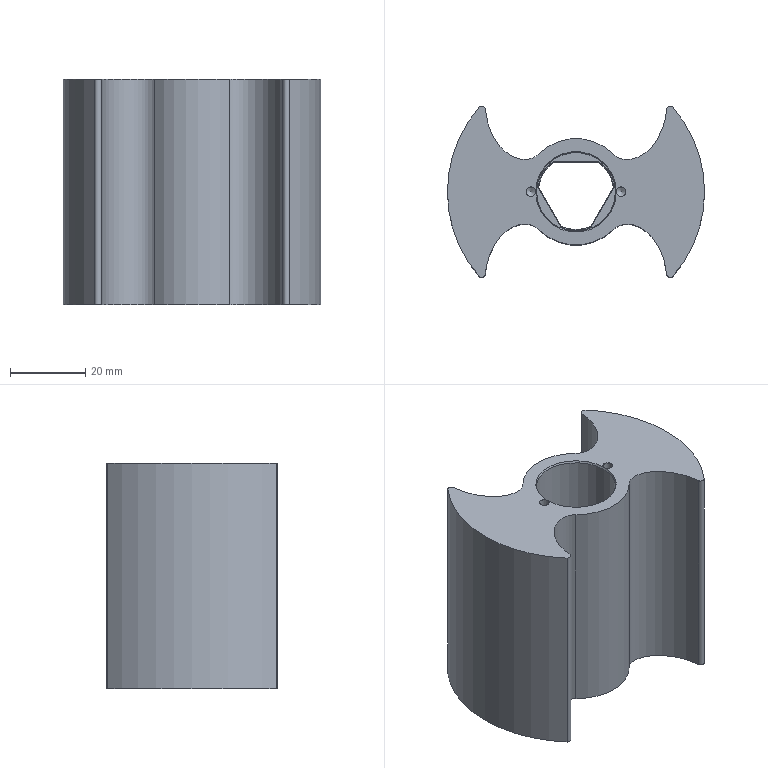NC program | NX | posted with a generic post | part box 68.489 x 45.577 x 60 mm
Whole program:
N10 G17 G21 G94 G90
(DRILLING_COPY_1 , TOOL : ZXZ)
N12 T01 M6
N14 G54
N16 G17 G0 G90 X-12. Y0. S5000 M3
N18 G43 Z30. H1
N20 G94 G81 G98 Z-1. F250. R3.
N22 X12.
N24 G80
N26 G0 X12. Y0. Z30.
N28 M5
(DRILLING_COPY_1_COPY , TOOL : 2.5ZT)
N30 T12 M6
N32 G54
N34 G17 G0 G90 X-12. Y0. S2000 M3
N36 G43 Z30. H12
N38 G94 G83 G98 Z-4.751 F120. Q2. R3.
N40 X12.
N42 G80
N44 G0 X12. Y0. Z30.
N46 M5
(ZLEVEL_PROFILE_COPY_1 , TOOL : D12)
N48 M6
N50 G54
N52 G17 G0 G90 X-0.209 Y-3.338 S3000 M3
N54 G43 Z30. H12
N56 Z-12.2
N58 G94 G1 X0. Y-3.7 Z-12.211 F1000.
N60 X3.204 Y1.85 Z-12.379
N62 X-3.204 Z-12.547
N64 X0. Y-3.7 Z-12.714
N66 X3.204 Y1.85 Z-12.882
N68 X-3.204 Z-13.05
N70 X0. Y-3.7 Z-13.218
N72 X3.204 Y1.85 Z-13.386
N74 X-3.204 Z-13.553
N76 X0. Y-3.7 Z-13.721
N78 X3.204 Y1.85 Z-13.889
N80 X-3.204 Z-14.057
N82 X0. Y-3.7 Z-14.225
N84 X3.204 Y1.85 Z-14.393
N86 X-3.204 Z-14.56
N88 X0. Y-3.7 Z-14.728
N90 X3.204 Y1.85 Z-14.896
N92 X-3.204 Z-15.064
N94 X0. Y-3.7 Z-15.232
N96 X3.204 Y1.85 Z-15.399
N98 X-3.204 F1800.
N100 X0. Y-3.7
N102 X3.204 Y1.85
N104 X-3.143 Z-15.51
N106 X-3.023 Y1.536 Z-15.518
N108 X-0.696 Y-2.495 Z-15.599
N110 X0. Y-3.7
N112 X3.204 Y1.85
N114 X-3.143 Z-15.71
N116 X-3.023 Y1.536 Z-15.717
N118 X-0.696 Y-2.495 Z-15.798
N120 X0. Y-3.7
N122 X3.204 Y1.85
N124 X-3.143 Z-15.909
N126 X-3.023 Y1.536 Z-15.916
N128 X-0.696 Y-2.495 Z-15.998
N130 X0. Y-3.7
N132 X3.204 Y1.85
N134 X-3.143 Z-16.109
N136 X-3.023 Y1.536 Z-16.116
N138 X-0.696 Y-2.495 Z-16.197
N140 X0. Y-3.7
N142 X3.204 Y1.85
N144 X-3.143 Z-16.308
N146 X-3.023 Y1.536 Z-16.315
N148 X-0.696 Y-2.495 Z-16.397
N150 X0. Y-3.7
N152 X3.204 Y1.85
N154 X-3.143 Z-16.507
N156 X-3.023 Y1.536 Z-16.515
N158 X-0.696 Y-2.495 Z-16.596
N160 X0. Y-3.7
N162 X3.204 Y1.85
N164 X-3.143 Z-16.707
N166 X-3.023 Y1.536 Z-16.714
N168 X-0.696 Y-2.495 Z-16.795
N170 X0. Y-3.7
N172 X3.204 Y1.85
N174 X-3.143 Z-16.906
N176 X-3.023 Y1.536 Z-16.914
N178 X-0.696 Y-2.495 Z-16.995
N180 X0. Y-3.7
N182 X3.204 Y1.85
N184 X-3.143 Z-17.106
N186 X-3.023 Y1.536 Z-17.113
N188 X-0.696 Y-2.495 Z-17.194
N190 X0. Y-3.7
N192 X3.204 Y1.85
N194 X-3.143 Z-17.305
N196 X-3.023 Y1.536 Z-17.313
N198 X-0.696 Y-2.495 Z-17.394
N200 X0. Y-3.7
N202 X3.204 Y1.85
N204 X-3.143 Z-17.505
N206 X-3.023 Y1.536 Z-17.512
N208 X-0.696 Y-2.495 Z-17.593
N210 X0. Y-3.7
N212 X3.204 Y1.85
N214 X-3.143 Z-17.704
N216 X-3.023 Y1.536 Z-17.711
N218 X-0.696 Y-2.495 Z-17.793
N220 X0. Y-3.7
N222 X3.204 Y1.85
N224 X-3.143 Z-17.903
N226 X-3.023 Y1.536 Z-17.911
N228 X-0.696 Y-2.495 Z-17.992
N230 X0. Y-3.7
N232 X3.204 Y1.85
N234 X-3.143 Z-18.103
N236 X-3.023 Y1.536 Z-18.11
N238 X-0.696 Y-2.495 Z-18.192
N240 X0. Y-3.7
N242 X3.204 Y1.85
N244 X-3.143 Z-18.302
N246 X-3.023 Y1.536 Z-18.31
N248 X-0.696 Y-2.495 Z-18.391
N250 X0. Y-3.7
N252 X3.204 Y1.85
N254 X-3.143 Z-18.502
N256 X-3.023 Y1.536 Z-18.509
N258 X-0.696 Y-2.495 Z-18.59
N260 X0. Y-3.7
N262 X3.204 Y1.85
N264 X-3.143 Z-18.701
N266 X-3.023 Y1.536 Z-18.709
N268 X-0.696 Y-2.495 Z-18.79
N270 X0. Y-3.7
N272 X3.204 Y1.85
N274 X-3.143 Z-18.901
N276 X-3.023 Y1.536 Z-18.908
N278 X-0.696 Y-2.495 Z-18.989
N280 X0. Y-3.7
N282 X3.204 Y1.85
N284 X-3.143 Z-19.1
N286 X-3.023 Y1.536 Z-19.107
N288 X-0.696 Y-2.495 Z-19.189
N290 X0. Y-3.7
N292 X3.204 Y1.85
N294 X-3.143 Z-19.299
N296 X-3.023 Y1.536 Z-19.307
N298 X-0.696 Y-2.495 Z-19.388
N300 X0. Y-3.7
N302 X3.204 Y1.85
N304 X-3.143 Z-19.499
N306 X-3.023 Y1.536 Z-19.506
N308 X-0.696 Y-2.495 Z-19.588
N310 X0. Y-3.7
N312 X3.204 Y1.85
N314 X-3.143 Z-19.698
N316 X-3.023 Y1.536 Z-19.706
N318 X-0.696 Y-2.495 Z-19.787
N320 X0. Y-3.7
N322 X3.204 Y1.85
N324 X-3.143 Z-19.898
N326 X-3.023 Y1.536 Z-19.905
N328 X-0.696 Y-2.495 Z-19.986
N330 X0. Y-3.7
N332 X3.204 Y1.85
N334 X-3.143 Z-20.097
N336 X-3.023 Y1.536 Z-20.105
N338 X-0.696 Y-2.495 Z-20.186
N340 X0. Y-3.7
N342 X3.204 Y1.85
N344 X-3.143 Z-20.297
N346 X-3.023 Y1.536 Z-20.304
N348 X-0.696 Y-2.495 Z-20.385
N350 X0. Y-3.7
N352 X3.204 Y1.85
N354 X-3.143 Z-20.496
N356 X-3.023 Y1.536 Z-20.503
N358 X-0.696 Y-2.495 Z-20.585
N360 X0. Y-3.7
N362 X3.204 Y1.85
N364 X-3.143 Z-20.696
N366 X-3.023 Y1.536 Z-20.703
N368 X-0.696 Y-2.495 Z-20.784
N370 X0. Y-3.7
N372 X3.204 Y1.85
N374 X-3.143 Z-20.895
N376 X-3.023 Y1.536 Z-20.902
N378 X-0.696 Y-2.495 Z-20.984
N380 X0. Y-3.7
N382 X3.204 Y1.85
N384 X-3.143 Z-21.094
N386 X-3.023 Y1.536 Z-21.102
N388 X-0.696 Y-2.495 Z-21.183
N390 X0. Y-3.7
N392 X3.204 Y1.85
N394 X-3.143 Z-21.294
N396 X-3.023 Y1.536 Z-21.301
N398 X-0.696 Y-2.495 Z-21.382
N400 X0. Y-3.7
N402 X3.204 Y1.85
N404 X-3.143 Z-21.493
N406 X-3.023 Y1.536 Z-21.501
N408 X-0.696 Y-2.495 Z-21.582
N410 X0. Y-3.7
N412 X3.204 Y1.85
N414 X-3.143 Z-21.693
N416 X-3.023 Y1.536 Z-21.7
N418 X-0.696 Y-2.495 Z-21.781
N420 X0. Y-3.7
N422 X3.204 Y1.85
N424 X-3.143 Z-21.892
N426 X-3.023 Y1.536 Z-21.9
N428 X-0.696 Y-2.495 Z-21.981
N430 X0. Y-3.7
N432 X3.204 Y1.85
N434 X-3.143 Z-22.092
N436 X-3.023 Y1.536 Z-22.099
N438 X-0.696 Y-2.495 Z-22.18
N440 X0. Y-3.7
N442 X3.204 Y1.85
N444 X-3.143 Z-22.291
N446 X-3.023 Y1.536 Z-22.298
N448 X-0.696 Y-2.495 Z-22.38
N450 X0. Y-3.7
N452 X3.204 Y1.85
N454 X-3.143 Z-22.49
N456 X-3.023 Y1.536 Z-22.498
N458 X-0.696 Y-2.495 Z-22.579
N460 X0. Y-3.7
N462 X3.204 Y1.85
N464 X-3.143 Z-22.69
N466 X-3.023 Y1.536 Z-22.697
N468 X-0.696 Y-2.495 Z-22.779
N470 X0. Y-3.7
N472 X3.204 Y1.85
N474 X-3.143 Z-22.889
N476 X-3.023 Y1.536 Z-22.897
N478 X-0.696 Y-2.495 Z-22.978
N480 X0. Y-3.7
N482 X3.204 Y1.85
N484 X-3.143 Z-23.089
N486 X-3.023 Y1.536 Z-23.096
N488 X-0.696 Y-2.495 Z-23.177
N490 X0. Y-3.7
N492 X3.204 Y1.85
N494 X-3.143 Z-23.288
N496 X-3.023 Y1.536 Z-23.296
N498 X-0.696 Y-2.495 Z-23.377
N500 X0. Y-3.7
N502 X3.204 Y1.85
N504 X-3.143 Z-23.488
N506 X-3.023 Y1.536 Z-23.495
N508 X-0.696 Y-2.495 Z-23.576
N510 X0. Y-3.7
N512 X3.204 Y1.85
N514 X-3.143 Z-23.687
N516 X-3.023 Y1.536 Z-23.694
N518 X-0.696 Y-2.495 Z-23.776
N520 X0. Y-3.7
N522 X3.204 Y1.85
N524 X-3.143 Z-23.887
N526 X-3.023 Y1.536 Z-23.894
N528 X-0.696 Y-2.495 Z-23.975
N530 X0. Y-3.7
N532 X3.204 Y1.85
N534 X-3.143 Z-24.086
N536 X-3.023 Y1.536 Z-24.093
N538 X-0.696 Y-2.495 Z-24.175
N540 X0. Y-3.7
N542 X3.204 Y1.85
N544 X-3.143 Z-24.285
N546 X-3.023 Y1.536 Z-24.293
N548 X-0.696 Y-2.495 Z-24.374
N550 X0. Y-3.7
N552 X3.204 Y1.85
N554 X-3.143 Z-24.485
N556 X-3.023 Y1.536 Z-24.492
N558 X-0.696 Y-2.495 Z-24.573
N560 X0. Y-3.7
N562 X3.204 Y1.85
N564 X-3.143 Z-24.684
N566 X-3.023 Y1.536 Z-24.692
N568 X-0.696 Y-2.495 Z-24.773
N570 X0. Y-3.7
N572 X3.204 Y1.85
N574 X-3.143 Z-24.884
N576 X-3.023 Y1.536 Z-24.891
N578 X-0.696 Y-2.495 Z-24.972
N580 X0. Y-3.7
N582 X3.204 Y1.85
N584 X-3.143 Z-25.083
N586 X-3.023 Y1.536 Z-25.091
N588 X-0.696 Y-2.495 Z-25.172
N590 X0. Y-3.7
N592 X3.204 Y1.85
N594 X-3.143 Z-25.283
N596 X-3.023 Y1.536 Z-25.29
N598 X-0.696 Y-2.495 Z-25.371
N600 X0. Y-3.7
N602 X3.204 Y1.85
N604 X-3.143 Z-25.482
N606 X-3.023 Y1.536 Z-25.489
N608 X-0.696 Y-2.495 Z-25.571
N610 X0. Y-3.7
N612 X3.204 Y1.85
N614 X-3.143 Z-25.681
N616 X-3.023 Y1.536 Z-25.689
N618 X-0.696 Y-2.495 Z-25.77
N620 X0. Y-3.7
N622 X3.204 Y1.85
N624 X-3.143 Z-25.881
N626 X-3.023 Y1.536 Z-25.888
N628 X-0.696 Y-2.495 Z-25.969
N630 X0. Y-3.7
N632 X3.204 Y1.85
N634 X-3.143 Z-26.08
N636 X-3.023 Y1.536 Z-26.088
N638 X-0.696 Y-2.495 Z-26.169
N640 X0. Y-3.7
N642 X3.204 Y1.85
N644 X-3.143 Z-26.28
N646 X-3.023 Y1.536 Z-26.287
N648 X-0.696 Y-2.495 Z-26.368
N650 X0. Y-3.7
N652 X3.204 Y1.85
N654 X-3.143 Z-26.479
N656 X-3.023 Y1.536 Z-26.487
N658 X-0.696 Y-2.495 Z-26.568
N660 X0. Y-3.7
N662 X3.204 Y1.85
N664 X-3.143 Z-26.679
N666 X-3.023 Y1.536 Z-26.686
N668 X-0.696 Y-2.495 Z-26.767
N670 X0. Y-3.7
N672 X3.204 Y1.85
N674 X-3.143 Z-26.878
N676 X-3.023 Y1.536 Z-26.885
N678 X-0.696 Y-2.495 Z-26.967
N680 X0. Y-3.7
N682 X3.204 Y1.85
N684 X-3.143 Z-27.077
N686 X-3.023 Y1.536 Z-27.085
N688 X-0.696 Y-2.495 Z-27.166
N690 X0. Y-3.7
N692 X3.204 Y1.85
N694 X-3.143 Z-27.277
N696 X-3.023 Y1.536 Z-27.284
N698 X-0.696 Y-2.495 Z-27.366
N700 X0. Y-3.7
N702 X3.204 Y1.85
N704 X-3.143 Z-27.476
N706 X-3.023 Y1.536 Z-27.484
N708 X-0.696 Y-2.495 Z-27.565
N710 X0. Y-3.7
N712 X3.204 Y1.85
N714 X-3.143 Z-27.676
N716 X-3.023 Y1.536 Z-27.683
N718 X-0.696 Y-2.495 Z-27.764
N720 X0. Y-3.7
N722 X3.204 Y1.85
N724 X-3.143 Z-27.875
N726 X-3.023 Y1.536 Z-27.883
N728 X-0.696 Y-2.495 Z-27.964
N730 X0. Y-3.7
N732 X3.204 Y1.85
N734 X-3.143 Z-28.075
N736 X-3.023 Y1.536 Z-28.082
N738 X-0.696 Y-2.495 Z-28.163
N740 X0. Y-3.7
N742 X3.204 Y1.85
N744 X-3.143 Z-28.274
N746 X-3.023 Y1.536 Z-28.281
N748 X-0.696 Y-2.495 Z-28.363
N750 X0. Y-3.7
N752 X3.204 Y1.85
N754 X-3.143 Z-28.474
N756 X-3.023 Y1.536 Z-28.481
N758 X-0.696 Y-2.495 Z-28.562
N760 X0. Y-3.7
N762 X3.204 Y1.85
N764 X-3.143 Z-28.673
N766 X-3.023 Y1.536 Z-28.68
N768 X-0.696 Y-2.495 Z-28.762
N770 X0. Y-3.7
N772 X3.204 Y1.85
N774 X-3.143 Z-28.872
N776 X-3.023 Y1.536 Z-28.88
N778 X-0.696 Y-2.495 Z-28.961
N780 X0. Y-3.7
N782 X3.204 Y1.85
N784 X-3.143 Z-29.072
N786 X-3.023 Y1.536 Z-29.079
N788 X-0.696 Y-2.495 Z-29.16
N790 X0. Y-3.7
N792 X3.204 Y1.85
N794 X-3.143 Z-29.271
N796 X-3.023 Y1.536 Z-29.279
N798 X-0.696 Y-2.495 Z-29.36
N800 X0. Y-3.7
N802 X3.204 Y1.85
N804 X-3.143 Z-29.471
N806 X-3.023 Y1.536 Z-29.478
N808 X-0.696 Y-2.495 Z-29.559
N810 X0. Y-3.7
N812 X3.204 Y1.85
N814 X-3.143 Z-29.67
N816 X-3.023 Y1.536 Z-29.678
N818 X-0.696 Y-2.495 Z-29.759
N820 X0. Y-3.7
N822 X3.204 Y1.85
N824 X-3.143 Z-29.87
N826 X-3.023 Y1.536 Z-29.877
N828 X-0.696 Y-2.495 Z-29.958
N830 X0. Y-3.7
N832 X3.204 Y1.85
N834 X-3.143 Z-30.069
N836 X-3.023 Y1.536 Z-30.076
N838 X-0.696 Y-2.495 Z-30.158
N840 X0. Y-3.7
N842 X3.204 Y1.85
N844 X-3.143 Z-30.268
N846 X-3.023 Y1.536 Z-30.276
N848 X-0.696 Y-2.495 Z-30.357
N850 X0. Y-3.7
N852 X3.204 Y1.85
N854 X-3.143 Z-30.468
N856 X-3.023 Y1.536 Z-30.475
N858 X-0.696 Y-2.495 Z-30.556
N860 X0. Y-3.7
N862 X3.204 Y1.85
N864 X-3.143 Z-30.667
N866 X-3.023 Y1.536 Z-30.675
N868 X-0.696 Y-2.495 Z-30.756
N870 X0. Y-3.7
N872 X3.204 Y1.85
N874 X-3.143 Z-30.867
N876 X-3.023 Y1.536 Z-30.874
N878 X-0.696 Y-2.495 Z-30.955
N880 X0. Y-3.7
N882 X3.204 Y1.85
N884 X-3.143 Z-31.066
N886 X-3.023 Y1.536 Z-31.074
N888 X-0.696 Y-2.495 Z-31.155
N890 X0. Y-3.7
N892 X3.204 Y1.85
N894 X-3.143 Z-31.266
N896 X-3.023 Y1.536 Z-31.273
N898 X-0.696 Y-2.495 Z-31.354
N900 X0. Y-3.7
N902 X3.204 Y1.85
N904 X-3.143 Z-31.465
N906 X-3.023 Y1.536 Z-31.472
N908 X-0.696 Y-2.495 Z-31.554
N910 X0. Y-3.7
N912 X3.204 Y1.85
N914 X-3.143 Z-31.664
N916 X-3.023 Y1.536 Z-31.672
N918 X-0.696 Y-2.495 Z-31.753
N920 X0. Y-3.7
N922 X3.204 Y1.85
N924 X-3.143 Z-31.864
N926 X-3.023 Y1.536 Z-31.871
N928 X-0.696 Y-2.495 Z-31.953
N930 X0. Y-3.7
N932 X3.204 Y1.85
N934 X-3.143 Z-32.063
N936 X-3.023 Y1.536 Z-32.071
N938 X-0.696 Y-2.495 Z-32.152
N940 X0. Y-3.7
N942 X3.204 Y1.85
N944 X-3.143 Z-32.263
N946 X-3.023 Y1.536 Z-32.27
N948 X-0.696 Y-2.495 Z-32.351
N950 X0. Y-3.7
N952 X3.204 Y1.85
N954 X-3.143 Z-32.462
N956 X-3.023 Y1.536 Z-32.47
N958 X-0.696 Y-2.495 Z-32.551
N960 X0. Y-3.7
N962 X3.204 Y1.85
N964 X-3.143 Z-32.662
N966 X-3.023 Y1.536 Z-32.669
N968 X-0.696 Y-2.495 Z-32.75
N970 X0. Y-3.7
N972 X3.204 Y1.85
N974 X-3.143 Z-32.861
N976 X-3.023 Y1.536 Z-32.868
N978 X-0.696 Y-2.495 Z-32.95
N980 X0. Y-3.7
N982 X3.204 Y1.85
N984 X-3.143 Z-33.061
N986 X-3.023 Y1.536 Z-33.068
N988 X-0.696 Y-2.495 Z-33.149
N990 X0. Y-3.7
N992 X3.204 Y1.85
N994 X-3.143 Z-33.26
N996 X-3.023 Y1.536 Z-33.267
N998 X-0.696 Y-2.495 Z-33.349
N1000 X0. Y-3.7
N1002 X3.204 Y1.85
N1004 X-3.143 Z-33.459
N1006 X-3.023 Y1.536 Z-33.467
N1008 X-0.696 Y-2.495 Z-33.548
N1010 X0. Y-3.7
N1012 X3.204 Y1.85
N1014 X-3.143 Z-33.659
N1016 X-3.023 Y1.536 Z-33.666
N1018 X-0.696 Y-2.495 Z-33.747
N1020 X0. Y-3.7
N1022 X3.204 Y1.85
N1024 X-3.143 Z-33.858
N1026 X-3.023 Y1.536 Z-33.866
N1028 X-0.696 Y-2.495 Z-33.947
N1030 X0. Y-3.7
N1032 X3.204 Y1.85
N1034 X-3.143 Z-34.058
N1036 X-3.023 Y1.536 Z-34.065
N1038 X-0.696 Y-2.495 Z-34.146
N1040 X0. Y-3.7
N1042 X3.204 Y1.85
N1044 X-3.143 Z-34.257
N1046 X-3.023 Y1.536 Z-34.265
N1048 X-0.696 Y-2.495 Z-34.346
N1050 X0. Y-3.7
N1052 X3.204 Y1.85
N1054 X-3.143 Z-34.457
N1056 X-3.023 Y1.536 Z-34.464
N1058 X-0.696 Y-2.495 Z-34.545
N1060 X0. Y-3.7
N1062 X3.204 Y1.85
N1064 X-3.143 Z-34.656
N1066 X-3.023 Y1.536 Z-34.663
N1068 X-0.696 Y-2.495 Z-34.745
N1070 X0. Y-3.7
N1072 X3.204 Y1.85
N1074 X-3.143 Z-34.855
N1076 X-3.023 Y1.536 Z-34.863
N1078 X-0.696 Y-2.495 Z-34.944
N1080 X0. Y-3.7
N1082 X3.204 Y1.85
N1084 X-3.143 Z-35.055
N1086 X-3.023 Y1.536 Z-35.062
N1088 X-0.696 Y-2.495 Z-35.144
N1090 X0. Y-3.7
N1092 X3.204 Y1.85
N1094 X-3.143 Z-35.254
N1096 X-3.023 Y1.536 Z-35.262
N1098 X-0.696 Y-2.495 Z-35.343
N1100 X0. Y-3.7
N1102 X3.204 Y1.85
N1104 X-3.143 Z-35.454
N1106 X-3.023 Y1.536 Z-35.461
N1108 X-0.696 Y-2.495 Z-35.542
N1110 X0. Y-3.7
N1112 X3.204 Y1.85
N1114 X-3.143 Z-35.653
N1116 X-3.023 Y1.536 Z-35.661
N1118 X-0.696 Y-2.495 Z-35.742
N1120 X0. Y-3.7
N1122 X3.204 Y1.85
N1124 X-3.143 Z-35.853
N1126 X-3.023 Y1.536 Z-35.86
N1128 X-0.696 Y-2.495 Z-35.941
N1130 X0. Y-3.7
N1132 X3.204 Y1.85
N1134 X-3.143 Z-36.052
N1136 X-3.023 Y1.536 Z-36.059
N1138 X-0.696 Y-2.495 Z-36.141
N1140 X0. Y-3.7
N1142 X3.204 Y1.85
N1144 X-3.143 Z-36.251
N1146 X-3.023 Y1.536 Z-36.259
N1148 X-0.696 Y-2.495 Z-36.34
N1150 X0. Y-3.7
N1152 X3.204 Y1.85
N1154 X-3.143 Z-36.451
N1156 X-3.023 Y1.536 Z-36.458
N1158 X-0.696 Y-2.495 Z-36.54
N1160 X0. Y-3.7
N1162 X3.204 Y1.85
N1164 X-3.143 Z-36.65
N1166 X-3.023 Y1.536 Z-36.658
N1168 X-0.696 Y-2.495 Z-36.739
N1170 X0. Y-3.7
N1172 X3.204 Y1.85
N1174 X-3.143 Z-36.85
N1176 X-3.023 Y1.536 Z-36.857
N1178 X-0.696 Y-2.495 Z-36.938
N1180 X0. Y-3.7
N1182 X3.204 Y1.85
N1184 X-3.143 Z-37.049
N1186 X-3.023 Y1.536 Z-37.057
N1188 X-0.696 Y-2.495 Z-37.138
N1190 X0. Y-3.7
N1192 X3.204 Y1.85
N1194 X-3.143 Z-37.249
N1196 X-3.023 Y1.536 Z-37.256
N1198 X-0.696 Y-2.495 Z-37.337
N1200 X0. Y-3.7
N1202 X3.204 Y1.85
N1204 X-3.143 Z-37.448
N1206 X-3.023 Y1.536 Z-37.455
N1208 X-0.696 Y-2.495 Z-37.537
N1210 X0. Y-3.7
N1212 X3.204 Y1.85
N1214 X-3.143 Z-37.648
N1216 X-3.023 Y1.536 Z-37.655
N1218 X-0.696 Y-2.495 Z-37.736
N1220 X0. Y-3.7
N1222 X3.204 Y1.85
N1224 X-3.143 Z-37.847
N1226 X-3.023 Y1.536 Z-37.854
N1228 X-0.696 Y-2.495 Z-37.936
N1230 X0. Y-3.7
N1232 X3.204 Y1.85
N1234 X-3.143 Z-38.046
N1236 X-3.023 Y1.536 Z-38.054
N1238 X-0.696 Y-2.495 Z-38.135
N1240 X0. Y-3.7
N1242 X3.204 Y1.85
N1244 X-3.143 Z-38.246
N1246 X-3.023 Y1.536 Z-38.253
N1248 X-0.696 Y-2.495 Z-38.334
N1250 X0. Y-3.7
N1252 X3.204 Y1.85
N1254 X-3.143 Z-38.445
N1256 X-3.023 Y1.536 Z-38.453
N1258 X-0.696 Y-2.495 Z-38.534
N1260 X0. Y-3.7
N1262 X3.204 Y1.85
N1264 X-3.143 Z-38.645
N1266 X-3.023 Y1.536 Z-38.652
N1268 X-0.696 Y-2.495 Z-38.733
N1270 X0. Y-3.7
N1272 X3.204 Y1.85
N1274 X-3.143 Z-38.844
N1276 X-3.023 Y1.536 Z-38.852
N1278 X-0.696 Y-2.495 Z-38.933
N1280 X0. Y-3.7
N1282 X3.204 Y1.85
N1284 X-3.143 Z-39.044
N1286 X-3.023 Y1.536 Z-39.051
N1288 X-0.696 Y-2.495 Z-39.132
N1290 X0. Y-3.7
N1292 X3.204 Y1.85
N1294 X-3.143 Z-39.243
N1296 X-3.023 Y1.536 Z-39.25
N1298 X-0.696 Y-2.495 Z-39.332
N1300 X0. Y-3.7
N1302 X3.204 Y1.85
N1304 X-3.143 Z-39.442
N1306 X-3.023 Y1.536 Z-39.45
N1308 X-0.696 Y-2.495 Z-39.531
N1310 X0. Y-3.7
N1312 X3.204 Y1.85
N1314 X-3.143 Z-39.642
N1316 X-3.023 Y1.536 Z-39.649
N1318 X-0.696 Y-2.495 Z-39.731
N1320 X0. Y-3.7
N1322 X3.204 Y1.85
N1324 X-3.143 Z-39.841
N1326 X-3.023 Y1.536 Z-39.849
N1328 X-0.696 Y-2.495 Z-39.93
N1330 X0. Y-3.7
N1332 X3.204 Y1.85
N1334 X-3.143 Z-40.041
N1336 X-3.023 Y1.536 Z-40.048
N1338 X-0.696 Y-2.495 Z-40.129
N1340 X0. Y-3.7
N1342 X3.204 Y1.85
N1344 X-3.143 Z-40.24
N1346 X-3.023 Y1.536 Z-40.248
N1348 X-0.696 Y-2.495 Z-40.329
N1350 X0. Y-3.7
N1352 X3.204 Y1.85
N1354 X-3.143 Z-40.44
N1356 X-3.023 Y1.536 Z-40.447
N1358 X-0.696 Y-2.495 Z-40.528
N1360 X0. Y-3.7
N1362 X3.204 Y1.85
N1364 X-3.143 Z-40.639
N1366 X-3.023 Y1.536 Z-40.646
N1368 X-0.696 Y-2.495 Z-40.728
N1370 X0. Y-3.7
N1372 X3.204 Y1.85
N1374 X-3.143 Z-40.838
N1376 X-3.023 Y1.536 Z-40.846
N1378 X-0.696 Y-2.495 Z-40.927
N1380 X0. Y-3.7
N1382 X3.204 Y1.85
N1384 X-3.143 Z-41.038
N1386 X-3.023 Y1.536 Z-41.045
N1388 X-0.696 Y-2.495 Z-41.127
N1390 X0. Y-3.7
N1392 X3.204 Y1.85
N1394 X-3.143 Z-41.237
N1396 X-3.023 Y1.536 Z-41.245
N1398 X-0.696 Y-2.495 Z-41.326
N1400 X0. Y-3.7
N1402 X3.204 Y1.85
N1404 X-3.143 Z-41.437
N1406 X-3.023 Y1.536 Z-41.444
N1408 X-0.696 Y-2.495 Z-41.525
N1410 X0. Y-3.7
N1412 X3.204 Y1.85
N1414 X-3.143 Z-41.636
N1416 X-3.023 Y1.536 Z-41.644
N1418 X-0.696 Y-2.495 Z-41.725
N1420 X0. Y-3.7
N1422 X3.204 Y1.85
N1424 X-3.143 Z-41.836
N1426 X-3.023 Y1.536 Z-41.843
N1428 X-0.696 Y-2.495 Z-41.924
N1430 X0. Y-3.7
N1432 X3.204 Y1.85
N1434 X-3.143 Z-42.035
N1436 X-3.023 Y1.536 Z-42.042
N1438 X-0.696 Y-2.495 Z-42.124
N1440 X0. Y-3.7
N1442 X3.204 Y1.85
N1444 X-3.143 Z-42.235
N1446 X-3.023 Y1.536 Z-42.242
N1448 X-0.696 Y-2.495 Z-42.323
N1450 X0. Y-3.7
N1452 X3.204 Y1.85
N1454 X-3.143 Z-42.434
N1456 X-3.023 Y1.536 Z-42.441
N1458 X-0.696 Y-2.495 Z-42.523
N1460 X0. Y-3.7
N1462 X3.204 Y1.85
N1464 X-3.143 Z-42.633
N1466 X-3.023 Y1.536 Z-42.641
N1468 X-0.696 Y-2.495 Z-42.722
N1470 X0. Y-3.7
N1472 X3.204 Y1.85
N1474 X-3.143 Z-42.833
N1476 X-3.023 Y1.536 Z-42.84
N1478 X-0.696 Y-2.495 Z-42.921
N1480 X0. Y-3.7
N1482 X3.204 Y1.85
N1484 X-3.143 Z-43.032
N1486 X-3.023 Y1.536 Z-43.04
N1488 X-0.696 Y-2.495 Z-43.121
N1490 X0. Y-3.7
N1492 X3.204 Y1.85
N1494 X-3.143 Z-43.232
N1496 X-3.023 Y1.536 Z-43.239
N1498 X-0.696 Y-2.495 Z-43.32
N1500 X0. Y-3.7
N1502 X3.204 Y1.85
N1504 X-3.143 Z-43.431
N1506 X-3.023 Y1.536 Z-43.439
N1508 X-0.696 Y-2.495 Z-43.52
N1510 X0. Y-3.7
N1512 X3.204 Y1.85
N1514 X-3.143 Z-43.631
N1516 X-3.023 Y1.536 Z-43.638
N1518 X-0.696 Y-2.495 Z-43.719
N1520 X0. Y-3.7
N1522 X3.204 Y1.85
N1524 X-3.143 Z-43.83
N1526 X-3.023 Y1.536 Z-43.837
N1528 X-0.696 Y-2.495 Z-43.919
N1530 X0. Y-3.7
N1532 X3.204 Y1.85
N1534 X-3.143 Z-44.029
N1536 X-3.023 Y1.536 Z-44.037
N1538 X-0.696 Y-2.495 Z-44.118
N1540 X0. Y-3.7
N1542 X3.204 Y1.85
N1544 X-3.143 Z-44.229
N1546 X-3.023 Y1.536 Z-44.236
N1548 X-0.696 Y-2.495 Z-44.318
N1550 X0. Y-3.7
N1552 X3.204 Y1.85
N1554 X-3.143 Z-44.428
N1556 X-3.023 Y1.536 Z-44.436
N1558 X-0.696 Y-2.495 Z-44.517
N1560 X0. Y-3.7
N1562 X3.204 Y1.85
N1564 X-3.143 Z-44.628
N1566 X-3.023 Y1.536 Z-44.635
N1568 X-0.696 Y-2.495 Z-44.716
N1570 X0. Y-3.7
N1572 X3.204 Y1.85
N1574 X-3.143 Z-44.827
N1576 X-3.023 Y1.536 Z-44.835
N1578 X-0.696 Y-2.495 Z-44.916
N1580 X0. Y-3.7
N1582 X3.204 Y1.85
N1584 X-3.143 Z-45.027
N1586 X-3.023 Y1.536 Z-45.034
N1588 X-0.696 Y-2.495 Z-45.115
N1590 X0. Y-3.7
N1592 X3.204 Y1.85
N1594 X-3.143 Z-45.226
N1596 X-3.023 Y1.536 Z-45.233
N1598 X-0.696 Y-2.495 Z-45.315
N1600 X0. Y-3.7
N1602 X3.204 Y1.85
N1604 X-3.143 Z-45.425
N1606 X-3.023 Y1.536 Z-45.433
N1608 X-0.696 Y-2.495 Z-45.514
N1610 X0. Y-3.7
N1612 X3.204 Y1.85
N1614 X-3.143 Z-45.625
N1616 X-3.023 Y1.536 Z-45.632
N1618 X-0.696 Y-2.495 Z-45.714
N1620 X0. Y-3.7
N1622 X3.204 Y1.85
N1624 X-3.143 Z-45.824
N1626 X-3.023 Y1.536 Z-45.832
N1628 X-0.696 Y-2.495 Z-45.913
N1630 X0. Y-3.7
N1632 X3.204 Y1.85
N1634 X-3.143 Z-46.024
N1636 X-3.023 Y1.536 Z-46.031
N1638 X-0.696 Y-2.495 Z-46.112
N1640 X0. Y-3.7
N1642 X3.204 Y1.85
N1644 X-3.143 Z-46.223
N1646 X-3.023 Y1.536 Z-46.231
N1648 X-0.696 Y-2.495 Z-46.312
N1650 X0. Y-3.7
N1652 X3.204 Y1.85
N1654 X-3.143 Z-46.423
N1656 X-3.023 Y1.536 Z-46.43
N1658 X-0.696 Y-2.495 Z-46.511
N1660 X0. Y-3.7
N1662 X3.204 Y1.85
N1664 X-3.143 Z-46.622
N1666 X-3.023 Y1.536 Z-46.629
N1668 X-0.696 Y-2.495 Z-46.711
N1670 X0. Y-3.7
N1672 X3.204 Y1.85
N1674 X-3.143 Z-46.822
N1676 X-3.023 Y1.536 Z-46.829
N1678 X-0.696 Y-2.495 Z-46.91
N1680 X0. Y-3.7
N1682 X3.204 Y1.85
N1684 X-3.143 Z-47.021
N1686 X-3.023 Y1.536 Z-47.028
N1688 X-0.696 Y-2.495 Z-47.11
N1690 X0. Y-3.7
N1692 X3.204 Y1.85
N1694 X-3.143 Z-47.22
N1696 X-3.023 Y1.536 Z-47.228
N1698 X-0.696 Y-2.495 Z-47.309
N1700 X0. Y-3.7
N1702 X3.204 Y1.85
N1704 X-3.143 Z-47.42
N1706 X-3.023 Y1.536 Z-47.427
N1708 X-0.696 Y-2.495 Z-47.508
N1710 X0. Y-3.7
N1712 X3.204 Y1.85
N1714 X-3.143 Z-47.619
N1716 X-3.023 Y1.536 Z-47.627
N1718 X-0.696 Y-2.495 Z-47.708
N1720 X0. Y-3.7
N1722 X3.204 Y1.85
N1724 X-3.143 Z-47.819
N1726 X-3.023 Y1.536 Z-47.826
N1728 X-0.696 Y-2.495 Z-47.907
N1730 X0. Y-3.7
N1732 X3.204 Y1.85
N1734 X-3.143 Z-48.018
N1736 X-3.023 Y1.536 Z-48.026
N1738 X-0.696 Y-2.495 Z-48.107
N1740 X0. Y-3.7
N1742 X3.204 Y1.85
N1744 X-3.143 Z-48.218
N1746 X-3.023 Y1.536 Z-48.225
N1748 X-0.696 Y-2.495 Z-48.306
N1750 X0. Y-3.7
N1752 X3.204 Y1.85
N1754 X-3.143 Z-48.417
N1756 X-3.023 Y1.536 Z-48.424
N1758 X-0.696 Y-2.495 Z-48.506
N1760 X0. Y-3.7
N1762 X3.204 Y1.85
N1764 X-3.143 Z-48.616
N1766 X-3.023 Y1.536 Z-48.624
N1768 X-0.696 Y-2.495 Z-48.705
N1770 X0. Y-3.7
N1772 X3.204 Y1.85
N1774 X-3.143 Z-48.816
N1776 X-3.023 Y1.536 Z-48.823
N1778 X-0.696 Y-2.495 Z-48.905
N1780 X0. Y-3.7
N1782 X3.204 Y1.85
N1784 X-3.143 Z-49.015
N1786 X-3.023 Y1.536 Z-49.023
N1788 X-0.696 Y-2.495 Z-49.104
N1790 X0. Y-3.7
N1792 X3.204 Y1.85
N1794 X-3.143 Z-49.215
N1796 X-3.023 Y1.536 Z-49.222
N1798 X-0.696 Y-2.495 Z-49.303
N1800 X0. Y-3.7
N1802 X3.204 Y1.85
N1804 X-3.143 Z-49.414
N1806 X-3.023 Y1.536 Z-49.422
N1808 X-0.696 Y-2.495 Z-49.503
N1810 X0. Y-3.7
N1812 X3.204 Y1.85
N1814 X-3.143 Z-49.614
N1816 X-3.023 Y1.536 Z-49.621
N1818 X-0.696 Y-2.495 Z-49.702
N1820 X0. Y-3.7
N1822 X3.204 Y1.85
N1824 X-3.143 Z-49.813
N1826 X-3.023 Y1.536 Z-49.82
N1828 X-0.696 Y-2.495 Z-49.902
N1830 X0. Y-3.7
N1832 X3.204 Y1.85
N1834 X-3.143 Z-50.012
N1836 X-3.023 Y1.536 Z-50.02
N1838 X-0.696 Y-2.495 Z-50.101
N1840 X0. Y-3.7
N1842 X3.204 Y1.85
N1844 X-3.143 Z-50.212
N1846 X-3.023 Y1.536 Z-50.219
N1848 X-0.696 Y-2.495 Z-50.301
N1850 X0. Y-3.7
N1852 X3.204 Y1.85
N1854 X-3.143 Z-50.411
N1856 X-3.023 Y1.536 Z-50.419
N1858 X-0.696 Y-2.495 Z-50.5
N1860 X0. Y-3.7
N1862 X3.204 Y1.85
N1864 X-3.204
N1866 X-0.696 Y-2.495
N1868 Z-47.5
N1870 G0 Z30.
(CUTTERCOMP12_1 , TOOL : D12)
N1872 X0.017 Y-1.402 S5000
N1874 Z-15.181
N1876 G1 Z-16.181 F1250.
N1878 G41 X0. Y-1.5 D12
N1880 Y-2.7
N1882 G3 X0. Y-3.9 R1.2
N1884 G1 X3.378 Y1.951
N1886 X3.335 Y1.95
N1888 X-3.335
N1890 X-3.378 Y1.951
N1892 X0. Y-3.9
N1894 G3 X0. Y-2.7 R1.2
N1896 G1 Y-1.5
N1898 G40
N1900 X-0.017 Y-1.402
N1902 Z-15.181
N1904 G0 Z30.
N1906 X0.017
N1908 Z-16.161
N1910 G1 Z-17.161
N1912 G41 X0. Y-1.5
N1914 Y-2.7
N1916 G3 X0. Y-3.9 R1.2
N1918 G1 X3.378 Y1.951
N1920 X3.335 Y1.95
N1922 X-3.335
N1924 X-3.378 Y1.951
N1926 X0. Y-3.9
N1928 G3 X0. Y-2.7 R1.2
N1930 G1 Y-1.5
N1932 G40
N1934 X-0.017 Y-1.402
N1936 Z-16.161
N1938 G0 Z30.
N1940 X0.017
N1942 Z-17.142
N1944 G1 Z-18.142
N1946 G41 X0. Y-1.5
N1948 Y-2.7
N1950 G3 X0. Y-3.9 R1.2
N1952 G1 X3.378 Y1.951
N1954 X3.335 Y1.95
N1956 X-3.335
N1958 X-3.378 Y1.951
N1960 X0. Y-3.9
N1962 G3 X0. Y-2.7 R1.2
N1964 G1 Y-1.5
N1966 G40
N1968 X-0.017 Y-1.402
N1970 Z-17.142
N1972 G0 Z30.
N1974 X0.017
N1976 Z-18.122
N1978 G1 Z-19.122
N1980 G41 X0. Y-1.5
N1982 Y-2.7
N1984 G3 X0. Y-3.9 R1.2
N1986 G1 X3.378 Y1.951
N1988 X3.335 Y1.95
N1990 X-3.335
N1992 X-3.378 Y1.951
N1994 X0. Y-3.9
N1996 G3 X0. Y-2.7 R1.2
N1998 G1 Y-1.5
N2000 G40
N2002 X-0.017 Y-1.402
N2004 Z-18.122
N2006 G0 Z30.
N2008 X0.017
N2010 Z-19.103
N2012 G1 Z-20.103
N2014 G41 X0. Y-1.5
N2016 Y-2.7
N2018 G3 X0. Y-3.9 R1.2
N2020 G1 X3.378 Y1.951
N2022 X3.335 Y1.95
N2024 X-3.335
N2026 X-3.378 Y1.951
N2028 X0. Y-3.9
N2030 G3 X0. Y-2.7 R1.2
N2032 G1 Y-1.5
N2034 G40
N2036 X-0.017 Y-1.402
N2038 Z-19.103
N2040 G0 Z30.
N2042 X0.017
N2044 Z-20.083
N2046 G1 Z-21.083
N2048 G41 X0. Y-1.5
N2050 Y-2.7
N2052 G3 X0. Y-3.9 R1.2
N2054 G1 X3.378 Y1.951
N2056 X3.335 Y1.95
N2058 X-3.335
N2060 X-3.378 Y1.951
N2062 X0. Y-3.9
N2064 G3 X0. Y-2.7 R1.2
N2066 G1 Y-1.5
N2068 G40
N2070 X-0.017 Y-1.402
N2072 Z-20.083
N2074 G0 Z30.
N2076 X0.017
N2078 Z-21.064
N2080 G1 Z-22.064
N2082 G41 X0. Y-1.5
N2084 Y-2.7
N2086 G3 X0. Y-3.9 R1.2
N2088 G1 X3.378 Y1.951
N2090 X3.335 Y1.95
N2092 X-3.335
N2094 X-3.378 Y1.951
N2096 X0. Y-3.9
N2098 G3 X0. Y-2.7 R1.2
N2100 G1 Y-1.5
N2102 G40
N2104 X-0.017 Y-1.402
N2106 Z-21.064
N2108 G0 Z30.
N2110 X0.017
N2112 Z-22.044
N2114 G1 Z-23.044
N2116 G41 X0. Y-1.5
N2118 Y-2.7
N2120 G3 X0. Y-3.9 R1.2
N2122 G1 X3.378 Y1.951
N2124 X3.335 Y1.95
N2126 X-3.335
N2128 X-3.378 Y1.951
N2130 X0. Y-3.9
N2132 G3 X0. Y-2.7 R1.2
N2134 G1 Y-1.5
N2136 G40
N2138 X-0.017 Y-1.402
N2140 Z-22.044
N2142 G0 Z30.
N2144 X0.017
N2146 Z-23.025
N2148 G1 Z-24.025
N2150 G41 X0. Y-1.5
N2152 Y-2.7
N2154 G3 X0. Y-3.9 R1.2
N2156 G1 X3.378 Y1.951
N2158 X3.335 Y1.95
N2160 X-3.335
N2162 X-3.378 Y1.951
N2164 X0. Y-3.9
N2166 G3 X0. Y-2.7 R1.2
N2168 G1 Y-1.5
N2170 G40
N2172 X-0.017 Y-1.402
N2174 Z-23.025
N2176 G0 Z30.
N2178 X0.017
N2180 Z-24.006
N2182 G1 Z-25.006
N2184 G41 X0. Y-1.5
N2186 Y-2.7
N2188 G3 X0. Y-3.9 R1.2
N2190 G1 X3.378 Y1.951
N2192 X3.335 Y1.95
N2194 X-3.335
N2196 X-3.378 Y1.951
N2198 X0. Y-3.9
N2200 G3 X0. Y-2.7 R1.2
N2202 G1 Y-1.5
N2204 G40
N2206 X-0.017 Y-1.402
N2208 Z-24.006
N2210 G0 Z30.
N2212 X0.017
N2214 Z-24.986
N2216 G1 Z-25.986
N2218 G41 X0. Y-1.5
N2220 Y-2.7
N2222 G3 X0. Y-3.9 R1.2
N2224 G1 X3.378 Y1.951
N2226 X3.335 Y1.95
N2228 X-3.335
N2230 X-3.378 Y1.951
N2232 X0. Y-3.9
N2234 G3 X0. Y-2.7 R1.2
N2236 G1 Y-1.5
N2238 G40
N2240 X-0.017 Y-1.402
N2242 Z-24.986
N2244 G0 Z30.
N2246 X0.017
N2248 Z-25.967
N2250 G1 Z-26.967
N2252 G41 X0. Y-1.5
N2254 Y-2.7
N2256 G3 X0. Y-3.9 R1.2
N2258 G1 X3.378 Y1.951
N2260 X3.335 Y1.95
N2262 X-3.335
N2264 X-3.378 Y1.951
N2266 X0. Y-3.9
N2268 G3 X0. Y-2.7 R1.2
N2270 G1 Y-1.5
N2272 G40
N2274 X-0.017 Y-1.402
N2276 Z-25.967
N2278 G0 Z30.
N2280 X0.017
N2282 Z-26.947
N2284 G1 Z-27.947
N2286 G41 X0. Y-1.5
N2288 Y-2.7
N2290 G3 X0. Y-3.9 R1.2
N2292 G1 X3.378 Y1.951
N2294 X3.335 Y1.95
N2296 X-3.335
N2298 X-3.378 Y1.951
N2300 X0. Y-3.9
N2302 G3 X0. Y-2.7 R1.2
N2304 G1 Y-1.5
N2306 G40
N2308 X-0.017 Y-1.402
N2310 Z-26.947
N2312 G0 Z30.
N2314 X0.017
N2316 Z-27.928
N2318 G1 Z-28.928
N2320 G41 X0. Y-1.5
N2322 Y-2.7
N2324 G3 X0. Y-3.9 R1.2
N2326 G1 X3.378 Y1.951
N2328 X3.335 Y1.95
N2330 X-3.335
N2332 X-3.378 Y1.951
N2334 X0. Y-3.9
N2336 G3 X0. Y-2.7 R1.2
N2338 G1 Y-1.5
N2340 G40
N2342 X-0.017 Y-1.402
N2344 Z-27.928
N2346 G0 Z30.
N2348 X0.017
N2350 Z-28.908
N2352 G1 Z-29.908
N2354 G41 X0. Y-1.5
N2356 Y-2.7
N2358 G3 X0. Y-3.9 R1.2
N2360 G1 X3.378 Y1.951
N2362 X3.335 Y1.95
N2364 X-3.335
N2366 X-3.378 Y1.951
N2368 X0. Y-3.9
N2370 G3 X0. Y-2.7 R1.2
N2372 G1 Y-1.5
N2374 G40
N2376 X-0.017 Y-1.402
N2378 Z-28.908
N2380 G0 Z30.
N2382 X0.017
N2384 Z-29.889
N2386 G1 Z-30.889
N2388 G41 X0. Y-1.5
N2390 Y-2.7
N2392 G3 X0. Y-3.9 R1.2
N2394 G1 X3.378 Y1.951
N2396 X3.335 Y1.95
N2398 X-3.335
N2400 X-3.378 Y1.951
N2402 X0. Y-3.9
N2404 G3 X0. Y-2.7 R1.2
N2406 G1 Y-1.5
N2408 G40
N2410 X-0.017 Y-1.402
N2412 Z-29.889
N2414 G0 Z30.
N2416 X0.017
N2418 Z-30.869
N2420 G1 Z-31.869
N2422 G41 X0. Y-1.5
N2424 Y-2.7
N2426 G3 X0. Y-3.9 R1.2
N2428 G1 X3.378 Y1.951
N2430 X3.335 Y1.95
N2432 X-3.335
N2434 X-3.378 Y1.951
N2436 X0. Y-3.9
N2438 G3 X0. Y-2.7 R1.2
N2440 G1 Y-1.5
N2442 G40
N2444 X-0.017 Y-1.402
N2446 Z-30.869
N2448 G0 Z30.
N2450 X0.017
N2452 Z-31.85
N2454 G1 Z-32.85
N2456 G41 X0. Y-1.5
N2458 Y-2.7
N2460 G3 X0. Y-3.9 R1.2
N2462 G1 X3.378 Y1.951
N2464 X3.335 Y1.95
N2466 X-3.335
N2468 X-3.378 Y1.951
N2470 X0. Y-3.9
N2472 G3 X0. Y-2.7 R1.2
N2474 G1 Y-1.5
N2476 G40
N2478 X-0.017 Y-1.402
N2480 Z-31.85
N2482 G0 Z30.
N2484 X0.017
N2486 Z-32.831
N2488 G1 Z-33.831
N2490 G41 X0. Y-1.5
N2492 Y-2.7
N2494 G3 X0. Y-3.9 R1.2
N2496 G1 X3.378 Y1.951
N2498 X3.335 Y1.95
N2500 X-3.335
N2502 X-3.378 Y1.951
N2504 X0. Y-3.9
N2506 G3 X0. Y-2.7 R1.2
N2508 G1 Y-1.5
N2510 G40
N2512 X-0.017 Y-1.402
N2514 Z-32.831
N2516 G0 Z30.
N2518 X0.017
N2520 Z-33.811
N2522 G1 Z-34.811
N2524 G41 X0. Y-1.5
N2526 Y-2.7
N2528 G3 X0. Y-3.9 R1.2
N2530 G1 X3.378 Y1.951
N2532 X3.335 Y1.95
N2534 X-3.335
N2536 X-3.378 Y1.951
N2538 X0. Y-3.9
N2540 G3 X0. Y-2.7 R1.2
N2542 G1 Y-1.5
N2544 G40
N2546 X-0.017 Y-1.402
N2548 Z-33.811
N2550 G0 Z30.
N2552 X0.017
N2554 Z-34.792
N2556 G1 Z-35.792
N2558 G41 X0. Y-1.5
N2560 Y-2.7
N2562 G3 X0. Y-3.9 R1.2
N2564 G1 X3.378 Y1.951
N2566 X3.335 Y1.95
N2568 X-3.335
N2570 X-3.378 Y1.951
N2572 X0. Y-3.9
N2574 G3 X0. Y-2.7 R1.2
N2576 G1 Y-1.5
N2578 G40
N2580 X-0.017 Y-1.402
N2582 Z-34.792
N2584 G0 Z30.
N2586 X0.017
N2588 Z-35.772
N2590 G1 Z-36.772
N2592 G41 X0. Y-1.5
N2594 Y-2.7
N2596 G3 X0. Y-3.9 R1.2
N2598 G1 X3.378 Y1.951
N2600 X3.335 Y1.95
N2602 X-3.335
N2604 X-3.378 Y1.951
N2606 X0. Y-3.9
N2608 G3 X0. Y-2.7 R1.2
N2610 G1 Y-1.5
N2612 G40
N2614 X-0.017 Y-1.402
N2616 Z-35.772
N2618 G0 Z30.
N2620 X0.017
N2622 Z-36.753
N2624 G1 Z-37.753
N2626 G41 X0. Y-1.5
N2628 Y-2.7
N2630 G3 X0. Y-3.9 R1.2
N2632 G1 X3.378 Y1.951
N2634 X3.335 Y1.95
N2636 X-3.335
N2638 X-3.378 Y1.951
N2640 X0. Y-3.9
N2642 G3 X0. Y-2.7 R1.2
N2644 G1 Y-1.5
N2646 G40
N2648 X-0.017 Y-1.402
N2650 Z-36.753
N2652 G0 Z30.
N2654 X0.017
N2656 Z-37.733
N2658 G1 Z-38.733
N2660 G41 X0. Y-1.5
N2662 Y-2.7
N2664 G3 X0. Y-3.9 R1.2
N2666 G1 X3.378 Y1.951
N2668 X3.335 Y1.95
N2670 X-3.335
N2672 X-3.378 Y1.951
N2674 X0. Y-3.9
N2676 G3 X0. Y-2.7 R1.2
N2678 G1 Y-1.5
N2680 G40
N2682 X-0.017 Y-1.402
N2684 Z-37.733
N2686 G0 Z30.
N2688 X0.017
N2690 Z-38.714
N2692 G1 Z-39.714
N2694 G41 X0. Y-1.5
N2696 Y-2.7
N2698 G3 X0. Y-3.9 R1.2
N2700 G1 X3.378 Y1.951
N2702 X3.335 Y1.95
N2704 X-3.335
N2706 X-3.378 Y1.951
N2708 X0. Y-3.9
N2710 G3 X0. Y-2.7 R1.2
N2712 G1 Y-1.5
N2714 G40
N2716 X-0.017 Y-1.402
N2718 Z-38.714
N2720 G0 Z30.
N2722 X0.017
N2724 Z-39.694
N2726 G1 Z-40.694
N2728 G41 X0. Y-1.5
N2730 Y-2.7
N2732 G3 X0. Y-3.9 R1.2
N2734 G1 X3.378 Y1.951
N2736 X3.335 Y1.95
N2738 X-3.335
N2740 X-3.378 Y1.951
N2742 X0. Y-3.9
N2744 G3 X0. Y-2.7 R1.2
N2746 G1 Y-1.5
N2748 G40
N2750 X-0.017 Y-1.402
N2752 Z-39.694
N2754 G0 Z30.
N2756 X0.017
N2758 Z-40.675
N2760 G1 Z-41.675
N2762 G41 X0. Y-1.5
N2764 Y-2.7
N2766 G3 X0. Y-3.9 R1.2
N2768 G1 X3.378 Y1.951
N2770 X3.335 Y1.95
N2772 X-3.335
N2774 X-3.378 Y1.951
N2776 X0. Y-3.9
N2778 G3 X0. Y-2.7 R1.2
N2780 G1 Y-1.5
N2782 G40
N2784 X-0.017 Y-1.402
N2786 Z-40.675
N2788 G0 Z30.
N2790 X0.017
N2792 Z-41.656
N2794 G1 Z-42.656
N2796 G41 X0. Y-1.5
N2798 Y-2.7
N2800 G3 X0. Y-3.9 R1.2
N2802 G1 X3.378 Y1.951
N2804 X3.335 Y1.95
N2806 X-3.335
N2808 X-3.378 Y1.951
N2810 X0. Y-3.9
N2812 G3 X0. Y-2.7 R1.2
N2814 G1 Y-1.5
N2816 G40
N2818 X-0.017 Y-1.402
N2820 Z-41.656
N2822 G0 Z30.
N2824 X0.017
N2826 Z-42.636
N2828 G1 Z-43.636
N2830 G41 X0. Y-1.5
N2832 Y-2.7
N2834 G3 X0. Y-3.9 R1.2
N2836 G1 X3.378 Y1.951
N2838 X3.335 Y1.95
N2840 X-3.335
N2842 X-3.378 Y1.951
N2844 X0. Y-3.9
N2846 G3 X0. Y-2.7 R1.2
N2848 G1 Y-1.5
N2850 G40
N2852 X-0.017 Y-1.402
N2854 Z-42.636
N2856 G0 Z30.
N2858 X0.017
N2860 Z-43.617
N2862 G1 Z-44.617
N2864 G41 X0. Y-1.5
N2866 Y-2.7
N2868 G3 X0. Y-3.9 R1.2
N2870 G1 X3.378 Y1.951
N2872 X3.335 Y1.95
N2874 X-3.335
N2876 X-3.378 Y1.951
N2878 X0. Y-3.9
N2880 G3 X0. Y-2.7 R1.2
N2882 G1 Y-1.5
N2884 G40
N2886 X-0.017 Y-1.402
N2888 Z-43.617
N2890 G0 Z30.
N2892 X0.017
N2894 Z-44.597
N2896 G1 Z-45.597
N2898 G41 X0. Y-1.5
N2900 Y-2.7
N2902 G3 X0. Y-3.9 R1.2
N2904 G1 X3.378 Y1.951
N2906 X3.335 Y1.95
N2908 X-3.335
N2910 X-3.378 Y1.951
N2912 X0. Y-3.9
N2914 G3 X0. Y-2.7 R1.2
N2916 G1 Y-1.5
N2918 G40
N2920 X-0.017 Y-1.402
N2922 Z-44.597
N2924 G0 Z30.
N2926 X0.017
N2928 Z-45.578
N2930 G1 Z-46.578
N2932 G41 X0. Y-1.5
N2934 Y-2.7
N2936 G3 X0. Y-3.9 R1.2
N2938 G1 X3.378 Y1.951
N2940 X3.335 Y1.95
N2942 X-3.335
N2944 X-3.378 Y1.951
N2946 X0. Y-3.9
N2948 G3 X0. Y-2.7 R1.2
N2950 G1 Y-1.5
N2952 G40
N2954 X-0.017 Y-1.402
N2956 Z-45.578
N2958 G0 Z30.
N2960 X0.017
N2962 Z-46.558
N2964 G1 Z-47.558
N2966 G41 X0. Y-1.5
N2968 Y-2.7
N2970 G3 X0. Y-3.9 R1.2
N2972 G1 X3.378 Y1.951
N2974 X3.335 Y1.95
N2976 X-3.335
N2978 X-3.378 Y1.951
N2980 X0. Y-3.9
N2982 G3 X0. Y-2.7 R1.2
N2984 G1 Y-1.5
N2986 G40
N2988 X-0.017 Y-1.402
N2990 Z-46.558
N2992 G0 Z30.
N2994 X0.017
N2996 Z-47.539
N2998 G1 Z-48.539
N3000 G41 X0. Y-1.5
N3002 Y-2.7
N3004 G3 X0. Y-3.9 R1.2
N3006 G1 X3.378 Y1.951
N3008 X3.335 Y1.95
N3010 X-3.335
N3012 X-3.378 Y1.951
N3014 X0. Y-3.9
N3016 G3 X0. Y-2.7 R1.2
N3018 G1 Y-1.5
N3020 G40
N3022 X-0.017 Y-1.402
N3024 Z-47.539
N3026 G0 Z30.
N3028 X0.017
N3030 Z-48.519
N3032 G1 Z-49.519
N3034 G41 X0. Y-1.5
N3036 Y-2.7
N3038 G3 X0. Y-3.9 R1.2
N3040 G1 X3.378 Y1.951
N3042 X3.335 Y1.95
N3044 X-3.335
N3046 X-3.378 Y1.951
N3048 X0. Y-3.9
N3050 G3 X0. Y-2.7 R1.2
N3052 G1 Y-1.5
N3054 G40
N3056 X-0.017 Y-1.402
N3058 Z-48.519
N3060 G0 Z30.
N3062 X0.017
N3064 Z-49.5
N3066 G1 Z-50.5
N3068 G41 X0. Y-1.5
N3070 Y-2.7
N3072 G3 X0. Y-3.9 R1.2
N3074 G1 X3.378 Y1.951
N3076 X3.335 Y1.95
N3078 X-3.335
N3080 X-3.378 Y1.951
N3082 X0. Y-3.9
N3084 G3 X0. Y-2.7 R1.2
N3086 G1 Y-1.5
N3088 G40
N3090 X-0.017 Y-1.402
N3092 Z-49.5
N3094 G0 Z30.
N3096 M5
N3098 M2